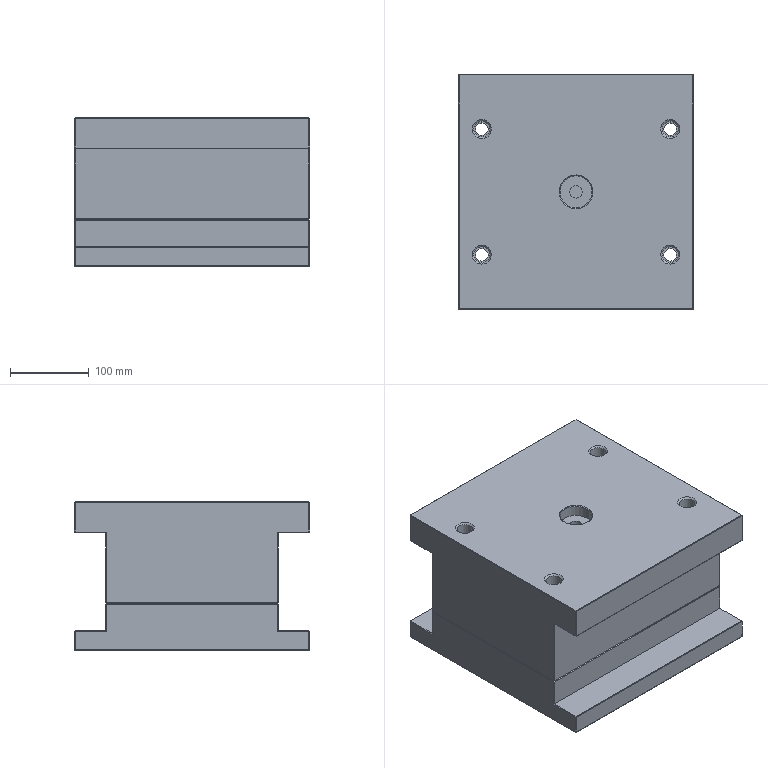NC program | NX | posted with a generic post | part box 300 x 300 x 190 mm
Lines 33427 to 34044 of 34829:
(HOLE_MILLING_COPY_1 , TOOL : D10C)
N66840 T10 M6
N66842 G54
N66844 G17 G0 G90 X-120. Y80. S2000 M3
N66846 G43 Z30. H10
N66848 Z0.5
N66850 G94 G3 X-118.555 Y78.555 R1.445 F800.
N66852 X-117.11 Y80. R1.445
N66854 X-117.11 Y80. Z0.3 I-2.89 J0.
N66856 X-117.11 Y80. Z0.1 I-2.89 J0.
N66858 X-117.11 Y80. Z-0.1 I-2.89 J0.
N66860 X-117.11 Y80. Z-0.3 I-2.89 J0.
N66862 X-117.11 Y80. Z-0.5 I-2.89 J0.
N66864 X-117.11 Y80. Z-0.7 I-2.89 J0.
N66866 X-117.11 Y80. Z-0.9 I-2.89 J0.
N66868 X-117.11 Y80. Z-1.1 I-2.89 J0.
N66870 X-117.11 Y80. Z-1.3 I-2.89 J0.
N66872 X-117.11 Y80. Z-1.5 I-2.89 J0.
N66874 X-117.11 Y80. Z-1.7 I-2.89 J0.
N66876 X-117.11 Y80. Z-1.9 I-2.89 J0.
N66878 X-117.11 Y80. Z-2.1 I-2.89 J0.
N66880 X-117.11 Y80. Z-2.3 I-2.89 J0.
N66882 X-117.11 Y80. Z-2.5 I-2.89 J0.
N66884 X-117.11 Y80. Z-2.7 I-2.89 J0.
N66886 X-117.11 Y80. Z-2.9 I-2.89 J0.
N66888 X-117.11 Y80. Z-3.1 I-2.89 J0.
N66890 X-117.11 Y80. Z-3.3 I-2.89 J0.
N66892 X-117.11 Y80. Z-3.5 I-2.89 J0.
N66894 X-117.11 Y80. Z-3.7 I-2.89 J0.
N66896 X-117.11 Y80. Z-3.9 I-2.89 J0.
N66898 X-117.11 Y80. Z-4.1 I-2.89 J0.
N66900 X-117.11 Y80. Z-4.3 I-2.89 J0.
N66902 X-117.11 Y80. Z-4.5 I-2.89 J0.
N66904 X-117.11 Y80. Z-4.7 I-2.89 J0.
N66906 X-117.11 Y80. Z-4.9 I-2.89 J0.
N66908 X-117.11 Y80. Z-5.1 I-2.89 J0.
N66910 X-117.11 Y80. Z-5.3 I-2.89 J0.
N66912 X-117.11 Y80. Z-5.5 I-2.89 J0.
N66914 X-117.11 Y80. Z-5.7 I-2.89 J0.
N66916 X-117.11 Y80. Z-5.9 I-2.89 J0.
N66918 X-117.11 Y80. Z-6.1 I-2.89 J0.
N66920 X-117.11 Y80. Z-6.3 I-2.89 J0.
N66922 X-117.11 Y80. Z-6.5 I-2.89 J0.
N66924 X-117.11 Y80. Z-6.7 I-2.89 J0.
N66926 X-117.11 Y80. Z-6.9 I-2.89 J0.
N66928 X-117.11 Y80. Z-7.1 I-2.89 J0.
N66930 X-117.11 Y80. Z-7.3 I-2.89 J0.
N66932 X-117.11 Y80. Z-7.5 I-2.89 J0.
N66934 X-117.11 Y80. Z-7.7 I-2.89 J0.
N66936 X-117.11 Y80. Z-7.9 I-2.89 J0.
N66938 X-117.11 Y80. Z-8.1 I-2.89 J0.
N66940 X-117.11 Y80. Z-8.3 I-2.89 J0.
N66942 X-117.11 Y80. Z-8.5 I-2.89 J0.
N66944 X-117.11 Y80. Z-8.7 I-2.89 J0.
N66946 X-117.11 Y80. Z-8.9 I-2.89 J0.
N66948 X-117.11 Y80. Z-9.1 I-2.89 J0.
N66950 X-117.11 Y80. Z-9.3 I-2.89 J0.
N66952 X-117.11 Y80. Z-9.5 I-2.89 J0.
N66954 X-117.11 Y80. Z-9.7 I-2.89 J0.
N66956 X-117.11 Y80. Z-9.9 I-2.89 J0.
N66958 X-117.11 Y80. Z-10.1 I-2.89 J0.
N66960 X-117.11 Y80. Z-10.3 I-2.89 J0.
N66962 X-117.11 Y80. Z-10.5 I-2.89 J0.
N66964 X-117.11 Y80. Z-10.7 I-2.89 J0.
N66966 X-117.11 Y80. Z-10.9 I-2.89 J0.
N66968 X-117.11 Y80. Z-11.1 I-2.89 J0.
N66970 X-117.11 Y80. Z-11.3 I-2.89 J0.
N66972 X-117.11 Y80. Z-11.5 I-2.89 J0.
N66974 X-117.11 Y80. Z-11.7 I-2.89 J0.
N66976 X-117.11 Y80. Z-11.9 I-2.89 J0.
N66978 X-117.11 Y80. Z-12.1 I-2.89 J0.
N66980 X-117.11 Y80. Z-12.3 I-2.89 J0.
N66982 X-117.11 Y80. Z-12.5 I-2.89 J0.
N66984 X-117.11 Y80. Z-12.7 I-2.89 J0.
N66986 X-117.11 Y80. Z-12.9 I-2.89 J0.
N66988 X-117.11 Y80. Z-13.1 I-2.89 J0.
N66990 X-117.11 Y80. Z-13.3 I-2.89 J0.
N66992 X-117.11 Y80. Z-13.5 I-2.89 J0.
N66994 X-117.11 Y80. Z-13.7 I-2.89 J0.
N66996 X-117.11 Y80. Z-13.9 I-2.89 J0.
N66998 X-117.11 Y80. Z-14.1 I-2.89 J0.
N67000 X-117.11 Y80. Z-14.3 I-2.89 J0.
N67002 X-117.11 Y80. Z-14.5 I-2.89 J0.
N67004 X-117.11 Y80. Z-14.7 I-2.89 J0.
N67006 X-117.11 Y80. Z-14.9 I-2.89 J0.
N67008 X-117.11 Y80. Z-15.1 I-2.89 J0.
N67010 X-117.11 Y80. Z-15.3 I-2.89 J0.
N67012 X-117.11 Y80. Z-15.5 I-2.89 J0.
N67014 X-117.11 Y80. Z-15.7 I-2.89 J0.
N67016 X-117.11 Y80. Z-15.9 I-2.89 J0.
N67018 X-117.11 Y80. Z-16.1 I-2.89 J0.
N67020 X-117.11 Y80. Z-16.3 I-2.89 J0.
N67022 X-117.11 Y80. Z-16.5 I-2.89 J0.
N67024 X-117.11 Y80. Z-16.7 I-2.89 J0.
N67026 X-117.11 Y80. Z-16.9 I-2.89 J0.
N67028 X-117.11 Y80. Z-17.1 I-2.89 J0.
N67030 X-117.11 Y80. Z-17.3 I-2.89 J0.
N67032 X-117.11 Y80. Z-17.5 I-2.89 J0.
N67034 X-117.11 Y80. Z-17.7 I-2.89 J0.
N67036 X-117.11 Y80. Z-17.9 I-2.89 J0.
N67038 X-117.11 Y80. Z-18.1 I-2.89 J0.
N67040 X-117.11 Y80. Z-18.3 I-2.89 J0.
N67042 X-117.11 Y80. Z-18.5 I-2.89 J0.
N67044 X-117.11 Y80. Z-18.7 I-2.89 J0.
N67046 X-117.11 Y80. Z-18.9 I-2.89 J0.
N67048 X-117.11 Y80. Z-19.1 I-2.89 J0.
N67050 X-117.11 Y80. Z-19.3 I-2.89 J0.
N67052 X-117.11 Y80. Z-19.5 I-2.89 J0.
N67054 X-117.11 Y80. Z-19.7 I-2.89 J0.
N67056 X-117.11 Y80. Z-19.9 I-2.89 J0.
N67058 X-117.11 Y80. Z-20.1 I-2.89 J0.
N67060 X-117.11 Y80. Z-20.3 I-2.89 J0.
N67062 X-117.11 Y80. Z-20.5 I-2.89 J0.
N67064 X-117.11 Y80. Z-20.7 I-2.89 J0.
N67066 X-117.11 Y80. Z-20.9 I-2.89 J0.
N67068 X-117.11 Y80. Z-21.1 I-2.89 J0.
N67070 X-117.11 Y80. Z-21.3 I-2.89 J0.
N67072 X-117.11 Y80. Z-21.5 I-2.89 J0.
N67074 X-117.11 Y80. Z-21.7 I-2.89 J0.
N67076 X-117.11 Y80. Z-21.9 I-2.89 J0.
N67078 X-117.11 Y80. Z-22.1 I-2.89 J0.
N67080 X-117.11 Y80. Z-22.3 I-2.89 J0.
N67082 X-117.11 Y80. Z-22.5 I-2.89 J0.
N67084 X-117.11 Y80. Z-22.7 I-2.89 J0.
N67086 X-117.11 Y80. Z-22.9 I-2.89 J0.
N67088 X-117.11 Y80. Z-23.1 I-2.89 J0.
N67090 X-117.11 Y80. Z-23.3 I-2.89 J0.
N67092 X-117.11 Y80. Z-23.5 I-2.89 J0.
N67094 X-117.11 Y80. Z-23.7 I-2.89 J0.
N67096 X-117.11 Y80. Z-23.9 I-2.89 J0.
N67098 X-117.11 Y80. Z-24.1 I-2.89 J0.
N67100 X-117.11 Y80. Z-24.3 I-2.89 J0.
N67102 X-117.11 Y80. Z-24.5 I-2.89 J0.
N67104 X-117.11 Y80. Z-24.7 I-2.89 J0.
N67106 X-117.11 Y80. Z-24.9 I-2.89 J0.
N67108 X-117.11 Y80. Z-25.1 I-2.89 J0.
N67110 X-117.11 Y80. Z-25.3 I-2.89 J0.
N67112 X-117.11 Y80. Z-25.5 I-2.89 J0.
N67114 X-117.11 Y80. Z-25.7 I-2.89 J0.
N67116 X-117.11 Y80. Z-25.9 I-2.89 J0.
N67118 X-117.11 Y80. Z-26.1 I-2.89 J0.
N67120 X-117.11 Y80. Z-26.3 I-2.89 J0.
N67122 X-117.11 Y80. Z-26.5 I-2.89 J0.
N67124 X-117.11 Y80. Z-26.7 I-2.89 J0.
N67126 X-117.11 Y80. Z-26.9 I-2.89 J0.
N67128 X-117.11 Y80. Z-27.1 I-2.89 J0.
N67130 X-117.11 Y80. Z-27.3 I-2.89 J0.
N67132 X-117.11 Y80. Z-27.5 I-2.89 J0.
N67134 X-117.11 Y80. Z-27.7 I-2.89 J0.
N67136 X-117.11 Y80. Z-27.9 I-2.89 J0.
N67138 X-117.11 Y80. Z-28.1 I-2.89 J0.
N67140 X-117.11 Y80. Z-28.3 I-2.89 J0.
N67142 X-117.11 Y80. Z-28.5 I-2.89 J0.
N67144 X-117.11 Y80. Z-28.7 I-2.89 J0.
N67146 X-117.11 Y80. Z-28.9 I-2.89 J0.
N67148 X-117.11 Y80. Z-29.1 I-2.89 J0.
N67150 X-117.11 Y80. Z-29.3 I-2.89 J0.
N67152 X-117.11 Y80. Z-29.5 I-2.89 J0.
N67154 X-117.11 Y80. Z-29.7 I-2.89 J0.
N67156 X-117.11 Y80. Z-29.9 I-2.89 J0.
N67158 X-117.11 Y80. Z-30.1 I-2.89 J0.
N67160 X-117.11 Y80. Z-30.3 I-2.89 J0.
N67162 X-117.11 Y80. Z-30.5 I-2.89 J0.
N67164 X-117.11 Y80. Z-30.7 I-2.89 J0.
N67166 X-117.11 Y80. Z-30.9 I-2.89 J0.
N67168 X-117.11 Y80. Z-31.1 I-2.89 J0.
N67170 X-117.11 Y80. Z-31.3 I-2.89 J0.
N67172 X-117.11 Y80. Z-31.5 I-2.89 J0.
N67174 X-117.11 Y80. Z-31.7 I-2.89 J0.
N67176 X-117.11 Y80. Z-31.9 I-2.89 J0.
N67178 X-117.11 Y80. Z-32.1 I-2.89 J0.
N67180 X-117.11 Y80. Z-32.3 I-2.89 J0.
N67182 X-117.11 Y80. Z-32.5 I-2.89 J0.
N67184 X-117.11 Y80. Z-32.7 I-2.89 J0.
N67186 X-117.11 Y80. Z-32.9 I-2.89 J0.
N67188 X-117.11 Y80. Z-33.1 I-2.89 J0.
N67190 X-117.11 Y80. Z-33.3 I-2.89 J0.
N67192 X-117.11 Y80. Z-33.5 I-2.89 J0.
N67194 X-117.11 Y80. Z-33.7 I-2.89 J0.
N67196 X-117.11 Y80. Z-33.9 I-2.89 J0.
N67198 X-117.11 Y80. Z-34.1 I-2.89 J0.
N67200 X-117.11 Y80. Z-34.3 I-2.89 J0.
N67202 X-117.11 Y80. Z-34.5 I-2.89 J0.
N67204 X-117.11 Y80. Z-34.7 I-2.89 J0.
N67206 X-117.11 Y80. Z-34.9 I-2.89 J0.
N67208 X-117.11 Y80. Z-35.1 I-2.89 J0.
N67210 X-117.11 Y80. Z-35.3 I-2.89 J0.
N67212 X-117.11 Y80. Z-35.5 I-2.89 J0.
N67214 X-117.11 Y80. Z-35.7 I-2.89 J0.
N67216 X-117.11 Y80. Z-35.9 I-2.89 J0.
N67218 X-117.11 Y80. Z-36.1 I-2.89 J0.
N67220 X-117.11 Y80. Z-36.3 I-2.89 J0.
N67222 X-117.11 Y80. Z-36.5 I-2.89 J0.
N67224 X-117.11 Y80. Z-36.7 I-2.89 J0.
N67226 X-117.11 Y80. Z-36.9 I-2.89 J0.
N67228 X-117.11 Y80. Z-37.1 I-2.89 J0.
N67230 X-117.11 Y80. Z-37.3 I-2.89 J0.
N67232 X-117.11 Y80. Z-37.5 I-2.89 J0.
N67234 X-117.11 Y80. Z-37.7 I-2.89 J0.
N67236 X-117.11 Y80. Z-37.9 I-2.89 J0.
N67238 X-117.11 Y80. Z-38.1 I-2.89 J0.
N67240 X-117.11 Y80. Z-38.3 I-2.89 J0.
N67242 X-117.11 Y80. Z-38.5 I-2.89 J0.
N67244 X-117.11 Y80. Z-38.7 I-2.89 J0.
N67246 X-117.11 Y80. Z-38.9 I-2.89 J0.
N67248 X-117.11 Y80. Z-39.1 I-2.89 J0.
N67250 X-117.11 Y80. Z-39.3 I-2.89 J0.
N67252 X-117.11 Y80. Z-39.5 I-2.89 J0.
N67254 X-117.11 Y80. Z-39.7 I-2.89 J0.
N67256 X-117.11 Y80. Z-39.9 I-2.89 J0.
N67258 X-117.11 Y80. Z-40.1 I-2.89 J0.
N67260 X-117.11 Y80. Z-40.3 I-2.89 J0.
N67262 X-117.11 Y80. Z-40.5 I-2.89 J0.
N67264 X-117.11 Y80. Z-40.7 I-2.89 J0.
N67266 X-117.11 Y80. Z-40.9 I-2.89 J0.
N67268 X-117.11 Y80. Z-41.1 I-2.89 J0.
N67270 X-117.11 Y80. Z-41.3 I-2.89 J0.
N67272 X-117.11 Y80. Z-41.5 I-2.89 J0.
N67274 X-117.11 Y80. Z-41.7 I-2.89 J0.
N67276 X-117.11 Y80. Z-41.9 I-2.89 J0.
N67278 X-117.11 Y80. Z-42.1 I-2.89 J0.
N67280 X-117.11 Y80. Z-42.3 I-2.89 J0.
N67282 X-117.11 Y80. Z-42.5 I-2.89 J0.
N67284 X-117.11 Y80. Z-42.7 I-2.89 J0.
N67286 X-117.11 Y80. Z-42.9 I-2.89 J0.
N67288 X-117.11 Y80. Z-43.1 I-2.89 J0.
N67290 X-117.11 Y80. Z-43.3 I-2.89 J0.
N67292 X-117.11 Y80. Z-43.5 I-2.89 J0.
N67294 X-117.11 Y80. Z-43.7 I-2.89 J0.
N67296 X-117.11 Y80. Z-43.9 I-2.89 J0.
N67298 X-117.11 Y80. Z-44.1 I-2.89 J0.
N67300 X-117.11 Y80. Z-44.3 I-2.89 J0.
N67302 X-117.11 Y80. Z-44.5 I-2.89 J0.
N67304 X-117.11 Y80. Z-44.7 I-2.89 J0.
N67306 X-117.11 Y80. Z-44.9 I-2.89 J0.
N67308 X-117.11 Y80. Z-45.1 I-2.89 J0.
N67310 X-117.11 Y80. Z-45.3 I-2.89 J0.
N67312 X-117.11 Y80. Z-45.5 I-2.89 J0.
N67314 X-117.11 Y80. Z-45.7 I-2.89 J0.
N67316 X-117.11 Y80. Z-45.9 I-2.89 J0.
N67318 X-117.11 Y80. Z-46.1 I-2.89 J0.
N67320 X-117.11 Y80. Z-46.3 I-2.89 J0.
N67322 X-117.11 Y80. Z-46.5 I-2.89 J0.
N67324 X-117.11 Y80. Z-46.7 I-2.89 J0.
N67326 X-117.11 Y80. Z-46.9 I-2.89 J0.
N67328 X-117.11 Y80. Z-47.1 I-2.89 J0.
N67330 X-117.11 Y80. Z-47.3 I-2.89 J0.
N67332 X-117.11 Y80. Z-47.5 I-2.89 J0.
N67334 X-117.11 Y80. Z-47.7 I-2.89 J0.
N67336 X-117.11 Y80. Z-47.9 I-2.89 J0.
N67338 X-117.11 Y80. Z-48.1 I-2.89 J0.
N67340 X-117.11 Y80. Z-48.3 I-2.89 J0.
N67342 X-117.11 Y80. Z-48.5 I-2.89 J0.
N67344 X-117.11 Y80. Z-48.7 I-2.89 J0.
N67346 X-117.11 Y80. Z-48.9 I-2.89 J0.
N67348 X-117.11 Y80. Z-49.1 I-2.89 J0.
N67350 X-117.11 Y80. Z-49.3 I-2.89 J0.
N67352 X-117.11 Y80. Z-49.5 I-2.89 J0.
N67354 X-117.11 Y80. Z-49.7 I-2.89 J0.
N67356 X-117.11 Y80. Z-49.9 I-2.89 J0.
N67358 X-117.11 Y80. Z-50.1 I-2.89 J0.
N67360 X-117.11 Y80. Z-50.3 I-2.89 J0.
N67362 X-117.11 Y80. Z-50.5 I-2.89 J0.
N67364 X-117.11 Y80. Z-50.7 I-2.89 J0.
N67366 X-117.11 Y80. Z-50.9 I-2.89 J0.
N67368 X-117.11 Y80. Z-51.1 I-2.89 J0.
N67370 X-117.11 Y80. Z-51.3 I-2.89 J0.
N67372 X-117.11 Y80. Z-51.5 I-2.89 J0.
N67374 X-117.11 Y80. Z-51.7 I-2.89 J0.
N67376 X-117.11 Y80. Z-51.9 I-2.89 J0.
N67378 X-117.11 Y80. Z-52.1 I-2.89 J0.
N67380 X-117.11 Y80. Z-52.3 I-2.89 J0.
N67382 X-117.11 Y80. Z-52.5 I-2.89 J0.
N67384 X-117.11 Y80. Z-52.7 I-2.89 J0.
N67386 X-117.11 Y80. Z-52.9 I-2.89 J0.
N67388 X-117.11 Y80. Z-53.1 I-2.89 J0.
N67390 X-117.11 Y80. Z-53.3 I-2.89 J0.
N67392 X-117.11 Y80. Z-53.5 I-2.89 J0.
N67394 X-117.11 Y80. Z-53.7 I-2.89 J0.
N67396 X-117.11 Y80. Z-53.9 I-2.89 J0.
N67398 X-117.11 Y80. Z-54.1 I-2.89 J0.
N67400 X-117.11 Y80. Z-54.3 I-2.89 J0.
N67402 X-117.11 Y80. Z-54.5 I-2.89 J0.
N67404 X-117.11 Y80. Z-54.7 I-2.89 J0.
N67406 X-117.11 Y80. Z-54.9 I-2.89 J0.
N67408 X-117.11 Y80. Z-55.1 I-2.89 J0.
N67410 X-117.11 Y80. Z-55.3 I-2.89 J0.
N67412 X-117.11 Y80. Z-55.5 I-2.89 J0.
N67414 X-117.11 Y80. Z-55.7 I-2.89 J0.
N67416 X-117.11 Y80. Z-55.9 I-2.89 J0.
N67418 X-117.11 Y80. Z-56.1 I-2.89 J0.
N67420 X-117.11 Y80. Z-56.3 I-2.89 J0.
N67422 X-117.11 Y80. Z-56.5 I-2.89 J0.
N67424 X-117.11 Y80. Z-56.7 I-2.89 J0.
N67426 X-117.11 Y80. Z-56.9 I-2.89 J0.
N67428 X-117.11 Y80. Z-57.1 I-2.89 J0.
N67430 X-117.11 Y80. Z-57.3 I-2.89 J0.
N67432 X-117.11 Y80. Z-57.5 I-2.89 J0.
N67434 X-117.11 Y80. Z-57.7 I-2.89 J0.
N67436 X-117.11 Y80. Z-57.9 I-2.89 J0.
N67438 X-117.11 Y80. Z-58.1 I-2.89 J0.
N67440 X-117.11 Y80. Z-58.3 I-2.89 J0.
N67442 X-117.11 Y80. Z-58.5 I-2.89 J0.
N67444 X-117.11 Y80. Z-58.7 I-2.89 J0.
N67446 X-117.11 Y80. Z-58.9 I-2.89 J0.
N67448 X-117.11 Y80. Z-59.1 I-2.89 J0.
N67450 X-117.11 Y80. Z-59.3 I-2.89 J0.
N67452 X-117.11 Y80. Z-59.5 I-2.89 J0.
N67454 X-117.11 Y80. Z-59.7 I-2.89 J0.
N67456 X-117.11 Y80. Z-59.9 I-2.89 J0.
N67458 X-122.89 Y80. Z-60. I-2.89 J0.
N67460 X-120. Y77.11 R2.89
N67462 X-122.89 Y80. R-2.89
N67464 X-121.445 Y78.555 R1.445
N67466 X-120. Y80. R1.445
N67468 G0 Z30.
N67470 Y-80.
N67472 Z0.5
N67474 G3 X-118.555 Y-81.445 R1.445
N67476 X-117.11 Y-80. R1.445
N67478 X-117.11 Y-80. Z0.3 I-2.89 J0.
N67480 X-117.11 Y-80. Z0.1 I-2.89 J0.
N67482 X-117.11 Y-80. Z-0.1 I-2.89 J0.
N67484 X-117.11 Y-80. Z-0.3 I-2.89 J0.
N67486 X-117.11 Y-80. Z-0.5 I-2.89 J0.
N67488 X-117.11 Y-80. Z-0.7 I-2.89 J0.
N67490 X-117.11 Y-80. Z-0.9 I-2.89 J0.
N67492 X-117.11 Y-80. Z-1.1 I-2.89 J0.
N67494 X-117.11 Y-80. Z-1.3 I-2.89 J0.
N67496 X-117.11 Y-80. Z-1.5 I-2.89 J0.
N67498 X-117.11 Y-80. Z-1.7 I-2.89 J0.
N67500 X-117.11 Y-80. Z-1.9 I-2.89 J0.
N67502 X-117.11 Y-80. Z-2.1 I-2.89 J0.
N67504 X-117.11 Y-80. Z-2.3 I-2.89 J0.
N67506 X-117.11 Y-80. Z-2.5 I-2.89 J0.
N67508 X-117.11 Y-80. Z-2.7 I-2.89 J0.
N67510 X-117.11 Y-80. Z-2.9 I-2.89 J0.
N67512 X-117.11 Y-80. Z-3.1 I-2.89 J0.
N67514 X-117.11 Y-80. Z-3.3 I-2.89 J0.
N67516 X-117.11 Y-80. Z-3.5 I-2.89 J0.
N67518 X-117.11 Y-80. Z-3.7 I-2.89 J0.
N67520 X-117.11 Y-80. Z-3.9 I-2.89 J0.
N67522 X-117.11 Y-80. Z-4.1 I-2.89 J0.
N67524 X-117.11 Y-80. Z-4.3 I-2.89 J0.
N67526 X-117.11 Y-80. Z-4.5 I-2.89 J0.
N67528 X-117.11 Y-80. Z-4.7 I-2.89 J0.
N67530 X-117.11 Y-80. Z-4.9 I-2.89 J0.
N67532 X-117.11 Y-80. Z-5.1 I-2.89 J0.
N67534 X-117.11 Y-80. Z-5.3 I-2.89 J0.
N67536 X-117.11 Y-80. Z-5.5 I-2.89 J0.
N67538 X-117.11 Y-80. Z-5.7 I-2.89 J0.
N67540 X-117.11 Y-80. Z-5.9 I-2.89 J0.
N67542 X-117.11 Y-80. Z-6.1 I-2.89 J0.
N67544 X-117.11 Y-80. Z-6.3 I-2.89 J0.
N67546 X-117.11 Y-80. Z-6.5 I-2.89 J0.
N67548 X-117.11 Y-80. Z-6.7 I-2.89 J0.
N67550 X-117.11 Y-80. Z-6.9 I-2.89 J0.
N67552 X-117.11 Y-80. Z-7.1 I-2.89 J0.
N67554 X-117.11 Y-80. Z-7.3 I-2.89 J0.
N67556 X-117.11 Y-80. Z-7.5 I-2.89 J0.
N67558 X-117.11 Y-80. Z-7.7 I-2.89 J0.
N67560 X-117.11 Y-80. Z-7.9 I-2.89 J0.
N67562 X-117.11 Y-80. Z-8.1 I-2.89 J0.
N67564 X-117.11 Y-80. Z-8.3 I-2.89 J0.
N67566 X-117.11 Y-80. Z-8.5 I-2.89 J0.
N67568 X-117.11 Y-80. Z-8.7 I-2.89 J0.
N67570 X-117.11 Y-80. Z-8.9 I-2.89 J0.
N67572 X-117.11 Y-80. Z-9.1 I-2.89 J0.
N67574 X-117.11 Y-80. Z-9.3 I-2.89 J0.
N67576 X-117.11 Y-80. Z-9.5 I-2.89 J0.
N67578 X-117.11 Y-80. Z-9.7 I-2.89 J0.
N67580 X-117.11 Y-80. Z-9.9 I-2.89 J0.
N67582 X-117.11 Y-80. Z-10.1 I-2.89 J0.
N67584 X-117.11 Y-80. Z-10.3 I-2.89 J0.
N67586 X-117.11 Y-80. Z-10.5 I-2.89 J0.
N67588 X-117.11 Y-80. Z-10.7 I-2.89 J0.
N67590 X-117.11 Y-80. Z-10.9 I-2.89 J0.
N67592 X-117.11 Y-80. Z-11.1 I-2.89 J0.
N67594 X-117.11 Y-80. Z-11.3 I-2.89 J0.
N67596 X-117.11 Y-80. Z-11.5 I-2.89 J0.
N67598 X-117.11 Y-80. Z-11.7 I-2.89 J0.
N67600 X-117.11 Y-80. Z-11.9 I-2.89 J0.
N67602 X-117.11 Y-80. Z-12.1 I-2.89 J0.
N67604 X-117.11 Y-80. Z-12.3 I-2.89 J0.
N67606 X-117.11 Y-80. Z-12.5 I-2.89 J0.
N67608 X-117.11 Y-80. Z-12.7 I-2.89 J0.
N67610 X-117.11 Y-80. Z-12.9 I-2.89 J0.
N67612 X-117.11 Y-80. Z-13.1 I-2.89 J0.
N67614 X-117.11 Y-80. Z-13.3 I-2.89 J0.
N67616 X-117.11 Y-80. Z-13.5 I-2.89 J0.
N67618 X-117.11 Y-80. Z-13.7 I-2.89 J0.
N67620 X-117.11 Y-80. Z-13.9 I-2.89 J0.
N67622 X-117.11 Y-80. Z-14.1 I-2.89 J0.
N67624 X-117.11 Y-80. Z-14.3 I-2.89 J0.
N67626 X-117.11 Y-80. Z-14.5 I-2.89 J0.
N67628 X-117.11 Y-80. Z-14.7 I-2.89 J0.
N67630 X-117.11 Y-80. Z-14.9 I-2.89 J0.
N67632 X-117.11 Y-80. Z-15.1 I-2.89 J0.
N67634 X-117.11 Y-80. Z-15.3 I-2.89 J0.
N67636 X-117.11 Y-80. Z-15.5 I-2.89 J0.
N67638 X-117.11 Y-80. Z-15.7 I-2.89 J0.
N67640 X-117.11 Y-80. Z-15.9 I-2.89 J0.
N67642 X-117.11 Y-80. Z-16.1 I-2.89 J0.
N67644 X-117.11 Y-80. Z-16.3 I-2.89 J0.
N67646 X-117.11 Y-80. Z-16.5 I-2.89 J0.
N67648 X-117.11 Y-80. Z-16.7 I-2.89 J0.
N67650 X-117.11 Y-80. Z-16.9 I-2.89 J0.
N67652 X-117.11 Y-80. Z-17.1 I-2.89 J0.
N67654 X-117.11 Y-80. Z-17.3 I-2.89 J0.
N67656 X-117.11 Y-80. Z-17.5 I-2.89 J0.
N67658 X-117.11 Y-80. Z-17.7 I-2.89 J0.
N67660 X-117.11 Y-80. Z-17.9 I-2.89 J0.
N67662 X-117.11 Y-80. Z-18.1 I-2.89 J0.
N67664 X-117.11 Y-80. Z-18.3 I-2.89 J0.
N67666 X-117.11 Y-80. Z-18.5 I-2.89 J0.
N67668 X-117.11 Y-80. Z-18.7 I-2.89 J0.
N67670 X-117.11 Y-80. Z-18.9 I-2.89 J0.
N67672 X-117.11 Y-80. Z-19.1 I-2.89 J0.
N67674 X-117.11 Y-80. Z-19.3 I-2.89 J0.
N67676 X-117.11 Y-80. Z-19.5 I-2.89 J0.
N67678 X-117.11 Y-80. Z-19.7 I-2.89 J0.
N67680 X-117.11 Y-80. Z-19.9 I-2.89 J0.
N67682 X-117.11 Y-80. Z-20.1 I-2.89 J0.
N67684 X-117.11 Y-80. Z-20.3 I-2.89 J0.
N67686 X-117.11 Y-80. Z-20.5 I-2.89 J0.
N67688 X-117.11 Y-80. Z-20.7 I-2.89 J0.
N67690 X-117.11 Y-80. Z-20.9 I-2.89 J0.
N67692 X-117.11 Y-80. Z-21.1 I-2.89 J0.
N67694 X-117.11 Y-80. Z-21.3 I-2.89 J0.
N67696 X-117.11 Y-80. Z-21.5 I-2.89 J0.
N67698 X-117.11 Y-80. Z-21.7 I-2.89 J0.
N67700 X-117.11 Y-80. Z-21.9 I-2.89 J0.
N67702 X-117.11 Y-80. Z-22.1 I-2.89 J0.
N67704 X-117.11 Y-80. Z-22.3 I-2.89 J0.
N67706 X-117.11 Y-80. Z-22.5 I-2.89 J0.
N67708 X-117.11 Y-80. Z-22.7 I-2.89 J0.
N67710 X-117.11 Y-80. Z-22.9 I-2.89 J0.
N67712 X-117.11 Y-80. Z-23.1 I-2.89 J0.
N67714 X-117.11 Y-80. Z-23.3 I-2.89 J0.
N67716 X-117.11 Y-80. Z-23.5 I-2.89 J0.
N67718 X-117.11 Y-80. Z-23.7 I-2.89 J0.
N67720 X-117.11 Y-80. Z-23.9 I-2.89 J0.
N67722 X-117.11 Y-80. Z-24.1 I-2.89 J0.
N67724 X-117.11 Y-80. Z-24.3 I-2.89 J0.
N67726 X-117.11 Y-80. Z-24.5 I-2.89 J0.
N67728 X-117.11 Y-80. Z-24.7 I-2.89 J0.
N67730 X-117.11 Y-80. Z-24.9 I-2.89 J0.
N67732 X-117.11 Y-80. Z-25.1 I-2.89 J0.
N67734 X-117.11 Y-80. Z-25.3 I-2.89 J0.
N67736 X-117.11 Y-80. Z-25.5 I-2.89 J0.
N67738 X-117.11 Y-80. Z-25.7 I-2.89 J0.
N67740 X-117.11 Y-80. Z-25.9 I-2.89 J0.
N67742 X-117.11 Y-80. Z-26.1 I-2.89 J0.
N67744 X-117.11 Y-80. Z-26.3 I-2.89 J0.
N67746 X-117.11 Y-80. Z-26.5 I-2.89 J0.
N67748 X-117.11 Y-80. Z-26.7 I-2.89 J0.
N67750 X-117.11 Y-80. Z-26.9 I-2.89 J0.
N67752 X-117.11 Y-80. Z-27.1 I-2.89 J0.
N67754 X-117.11 Y-80. Z-27.3 I-2.89 J0.
N67756 X-117.11 Y-80. Z-27.5 I-2.89 J0.
N67758 X-117.11 Y-80. Z-27.7 I-2.89 J0.
N67760 X-117.11 Y-80. Z-27.9 I-2.89 J0.
N67762 X-117.11 Y-80. Z-28.1 I-2.89 J0.
N67764 X-117.11 Y-80. Z-28.3 I-2.89 J0.
N67766 X-117.11 Y-80. Z-28.5 I-2.89 J0.
N67768 X-117.11 Y-80. Z-28.7 I-2.89 J0.
N67770 X-117.11 Y-80. Z-28.9 I-2.89 J0.
N67772 X-117.11 Y-80. Z-29.1 I-2.89 J0.
N67774 X-117.11 Y-80. Z-29.3 I-2.89 J0.
N67776 X-117.11 Y-80. Z-29.5 I-2.89 J0.
N67778 X-117.11 Y-80. Z-29.7 I-2.89 J0.
N67780 X-117.11 Y-80. Z-29.9 I-2.89 J0.
N67782 X-117.11 Y-80. Z-30.1 I-2.89 J0.
N67784 X-117.11 Y-80. Z-30.3 I-2.89 J0.
N67786 X-117.11 Y-80. Z-30.5 I-2.89 J0.
N67788 X-117.11 Y-80. Z-30.7 I-2.89 J0.
N67790 X-117.11 Y-80. Z-30.9 I-2.89 J0.
N67792 X-117.11 Y-80. Z-31.1 I-2.89 J0.
N67794 X-117.11 Y-80. Z-31.3 I-2.89 J0.
N67796 X-117.11 Y-80. Z-31.5 I-2.89 J0.
N67798 X-117.11 Y-80. Z-31.7 I-2.89 J0.
N67800 X-117.11 Y-80. Z-31.9 I-2.89 J0.
N67802 X-117.11 Y-80. Z-32.1 I-2.89 J0.
N67804 X-117.11 Y-80. Z-32.3 I-2.89 J0.
N67806 X-117.11 Y-80. Z-32.5 I-2.89 J0.
N67808 X-117.11 Y-80. Z-32.7 I-2.89 J0.
N67810 X-117.11 Y-80. Z-32.9 I-2.89 J0.
N67812 X-117.11 Y-80. Z-33.1 I-2.89 J0.
N67814 X-117.11 Y-80. Z-33.3 I-2.89 J0.
N67816 X-117.11 Y-80. Z-33.5 I-2.89 J0.
N67818 X-117.11 Y-80. Z-33.7 I-2.89 J0.
N67820 X-117.11 Y-80. Z-33.9 I-2.89 J0.
N67822 X-117.11 Y-80. Z-34.1 I-2.89 J0.
N67824 X-117.11 Y-80. Z-34.3 I-2.89 J0.
N67826 X-117.11 Y-80. Z-34.5 I-2.89 J0.
N67828 X-117.11 Y-80. Z-34.7 I-2.89 J0.
N67830 X-117.11 Y-80. Z-34.9 I-2.89 J0.
N67832 X-117.11 Y-80. Z-35.1 I-2.89 J0.
N67834 X-117.11 Y-80. Z-35.3 I-2.89 J0.
N67836 X-117.11 Y-80. Z-35.5 I-2.89 J0.
N67838 X-117.11 Y-80. Z-35.7 I-2.89 J0.
N67840 X-117.11 Y-80. Z-35.9 I-2.89 J0.
N67842 X-117.11 Y-80. Z-36.1 I-2.89 J0.
N67844 X-117.11 Y-80. Z-36.3 I-2.89 J0.
N67846 X-117.11 Y-80. Z-36.5 I-2.89 J0.
N67848 X-117.11 Y-80. Z-36.7 I-2.89 J0.
N67850 X-117.11 Y-80. Z-36.9 I-2.89 J0.
N67852 X-117.11 Y-80. Z-37.1 I-2.89 J0.
N67854 X-117.11 Y-80. Z-37.3 I-2.89 J0.
N67856 X-117.11 Y-80. Z-37.5 I-2.89 J0.
N67858 X-117.11 Y-80. Z-37.7 I-2.89 J0.
N67860 X-117.11 Y-80. Z-37.9 I-2.89 J0.
N67862 X-117.11 Y-80. Z-38.1 I-2.89 J0.
N67864 X-117.11 Y-80. Z-38.3 I-2.89 J0.
N67866 X-117.11 Y-80. Z-38.5 I-2.89 J0.
N67868 X-117.11 Y-80. Z-38.7 I-2.89 J0.
N67870 X-117.11 Y-80. Z-38.9 I-2.89 J0.
N67872 X-117.11 Y-80. Z-39.1 I-2.89 J0.
N67874 X-117.11 Y-80. Z-39.3 I-2.89 J0.
N67876 X-117.11 Y-80. Z-39.5 I-2.89 J0.
N67878 X-117.11 Y-80. Z-39.7 I-2.89 J0.
N67880 X-117.11 Y-80. Z-39.9 I-2.89 J0.
N67882 X-117.11 Y-80. Z-40.1 I-2.89 J0.
N67884 X-117.11 Y-80. Z-40.3 I-2.89 J0.
N67886 X-117.11 Y-80. Z-40.5 I-2.89 J0.
N67888 X-117.11 Y-80. Z-40.7 I-2.89 J0.
N67890 X-117.11 Y-80. Z-40.9 I-2.89 J0.
N67892 X-117.11 Y-80. Z-41.1 I-2.89 J0.
N67894 X-117.11 Y-80. Z-41.3 I-2.89 J0.
N67896 X-117.11 Y-80. Z-41.5 I-2.89 J0.
N67898 X-117.11 Y-80. Z-41.7 I-2.89 J0.
N67900 X-117.11 Y-80. Z-41.9 I-2.89 J0.
N67902 X-117.11 Y-80. Z-42.1 I-2.89 J0.
N67904 X-117.11 Y-80. Z-42.3 I-2.89 J0.
N67906 X-117.11 Y-80. Z-42.5 I-2.89 J0.
N67908 X-117.11 Y-80. Z-42.7 I-2.89 J0.
N67910 X-117.11 Y-80. Z-42.9 I-2.89 J0.
N67912 X-117.11 Y-80. Z-43.1 I-2.89 J0.
N67914 X-117.11 Y-80. Z-43.3 I-2.89 J0.
N67916 X-117.11 Y-80. Z-43.5 I-2.89 J0.
N67918 X-117.11 Y-80. Z-43.7 I-2.89 J0.
N67920 X-117.11 Y-80. Z-43.9 I-2.89 J0.
N67922 X-117.11 Y-80. Z-44.1 I-2.89 J0.
N67924 X-117.11 Y-80. Z-44.3 I-2.89 J0.
N67926 X-117.11 Y-80. Z-44.5 I-2.89 J0.
N67928 X-117.11 Y-80. Z-44.7 I-2.89 J0.
N67930 X-117.11 Y-80. Z-44.9 I-2.89 J0.
N67932 X-117.11 Y-80. Z-45.1 I-2.89 J0.
N67934 X-117.11 Y-80. Z-45.3 I-2.89 J0.
N67936 X-117.11 Y-80. Z-45.5 I-2.89 J0.
N67938 X-117.11 Y-80. Z-45.7 I-2.89 J0.
N67940 X-117.11 Y-80. Z-45.9 I-2.89 J0.
N67942 X-117.11 Y-80. Z-46.1 I-2.89 J0.
N67944 X-117.11 Y-80. Z-46.3 I-2.89 J0.
N67946 X-117.11 Y-80. Z-46.5 I-2.89 J0.
N67948 X-117.11 Y-80. Z-46.7 I-2.89 J0.
N67950 X-117.11 Y-80. Z-46.9 I-2.89 J0.
N67952 X-117.11 Y-80. Z-47.1 I-2.89 J0.
N67954 X-117.11 Y-80. Z-47.3 I-2.89 J0.
N67956 X-117.11 Y-80. Z-47.5 I-2.89 J0.
N67958 X-117.11 Y-80. Z-47.7 I-2.89 J0.
N67960 X-117.11 Y-80. Z-47.9 I-2.89 J0.
N67962 X-117.11 Y-80. Z-48.1 I-2.89 J0.
N67964 X-117.11 Y-80. Z-48.3 I-2.89 J0.
N67966 X-117.11 Y-80. Z-48.5 I-2.89 J0.
N67968 X-117.11 Y-80. Z-48.7 I-2.89 J0.
N67970 X-117.11 Y-80. Z-48.9 I-2.89 J0.
N67972 X-117.11 Y-80. Z-49.1 I-2.89 J0.
N67974 X-117.11 Y-80. Z-49.3 I-2.89 J0.
N67976 X-117.11 Y-80. Z-49.5 I-2.89 J0.
N67978 X-117.11 Y-80. Z-49.7 I-2.89 J0.
N67980 X-117.11 Y-80. Z-49.9 I-2.89 J0.
N67982 X-117.11 Y-80. Z-50.1 I-2.89 J0.
N67984 X-117.11 Y-80. Z-50.3 I-2.89 J0.
N67986 X-117.11 Y-80. Z-50.5 I-2.89 J0.
N67988 X-117.11 Y-80. Z-50.7 I-2.89 J0.
N67990 X-117.11 Y-80. Z-50.9 I-2.89 J0.
N67992 X-117.11 Y-80. Z-51.1 I-2.89 J0.
N67994 X-117.11 Y-80. Z-51.3 I-2.89 J0.
N67996 X-117.11 Y-80. Z-51.5 I-2.89 J0.
N67998 X-117.11 Y-80. Z-51.7 I-2.89 J0.
N68000 X-117.11 Y-80. Z-51.9 I-2.89 J0.
N68002 X-117.11 Y-80. Z-52.1 I-2.89 J0.
N68004 X-117.11 Y-80. Z-52.3 I-2.89 J0.
N68006 X-117.11 Y-80. Z-52.5 I-2.89 J0.
N68008 X-117.11 Y-80. Z-52.7 I-2.89 J0.
N68010 X-117.11 Y-80. Z-52.9 I-2.89 J0.
N68012 X-117.11 Y-80. Z-53.1 I-2.89 J0.
N68014 X-117.11 Y-80. Z-53.3 I-2.89 J0.
N68016 X-117.11 Y-80. Z-53.5 I-2.89 J0.
N68018 X-117.11 Y-80. Z-53.7 I-2.89 J0.
N68020 X-117.11 Y-80. Z-53.9 I-2.89 J0.
N68022 X-117.11 Y-80. Z-54.1 I-2.89 J0.
N68024 X-117.11 Y-80. Z-54.3 I-2.89 J0.
N68026 X-117.11 Y-80. Z-54.5 I-2.89 J0.
N68028 X-117.11 Y-80. Z-54.7 I-2.89 J0.
N68030 X-117.11 Y-80. Z-54.9 I-2.89 J0.
N68032 X-117.11 Y-80. Z-55.1 I-2.89 J0.
N68034 X-117.11 Y-80. Z-55.3 I-2.89 J0.
N68036 X-117.11 Y-80. Z-55.5 I-2.89 J0.
N68038 X-117.11 Y-80. Z-55.7 I-2.89 J0.
N68040 X-117.11 Y-80. Z-55.9 I-2.89 J0.
N68042 X-117.11 Y-80. Z-56.1 I-2.89 J0.
N68044 X-117.11 Y-80. Z-56.3 I-2.89 J0.
N68046 X-117.11 Y-80. Z-56.5 I-2.89 J0.
N68048 X-117.11 Y-80. Z-56.7 I-2.89 J0.
N68050 X-117.11 Y-80. Z-56.9 I-2.89 J0.
N68052 X-117.11 Y-80. Z-57.1 I-2.89 J0.
N68054 X-117.11 Y-80. Z-57.3 I-2.89 J0.
N68056 X-117.11 Y-80. Z-57.5 I-2.89 J0.
N68058 X-117.11 Y-80. Z-57.7 I-2.89 J0.
N68060 X-117.11 Y-80. Z-57.9 I-2.89 J0.
N68062 X-117.11 Y-80. Z-58.1 I-2.89 J0.
N68064 X-117.11 Y-80. Z-58.3 I-2.89 J0.
N68066 X-117.11 Y-80. Z-58.5 I-2.89 J0.
N68068 X-117.11 Y-80. Z-58.7 I-2.89 J0.